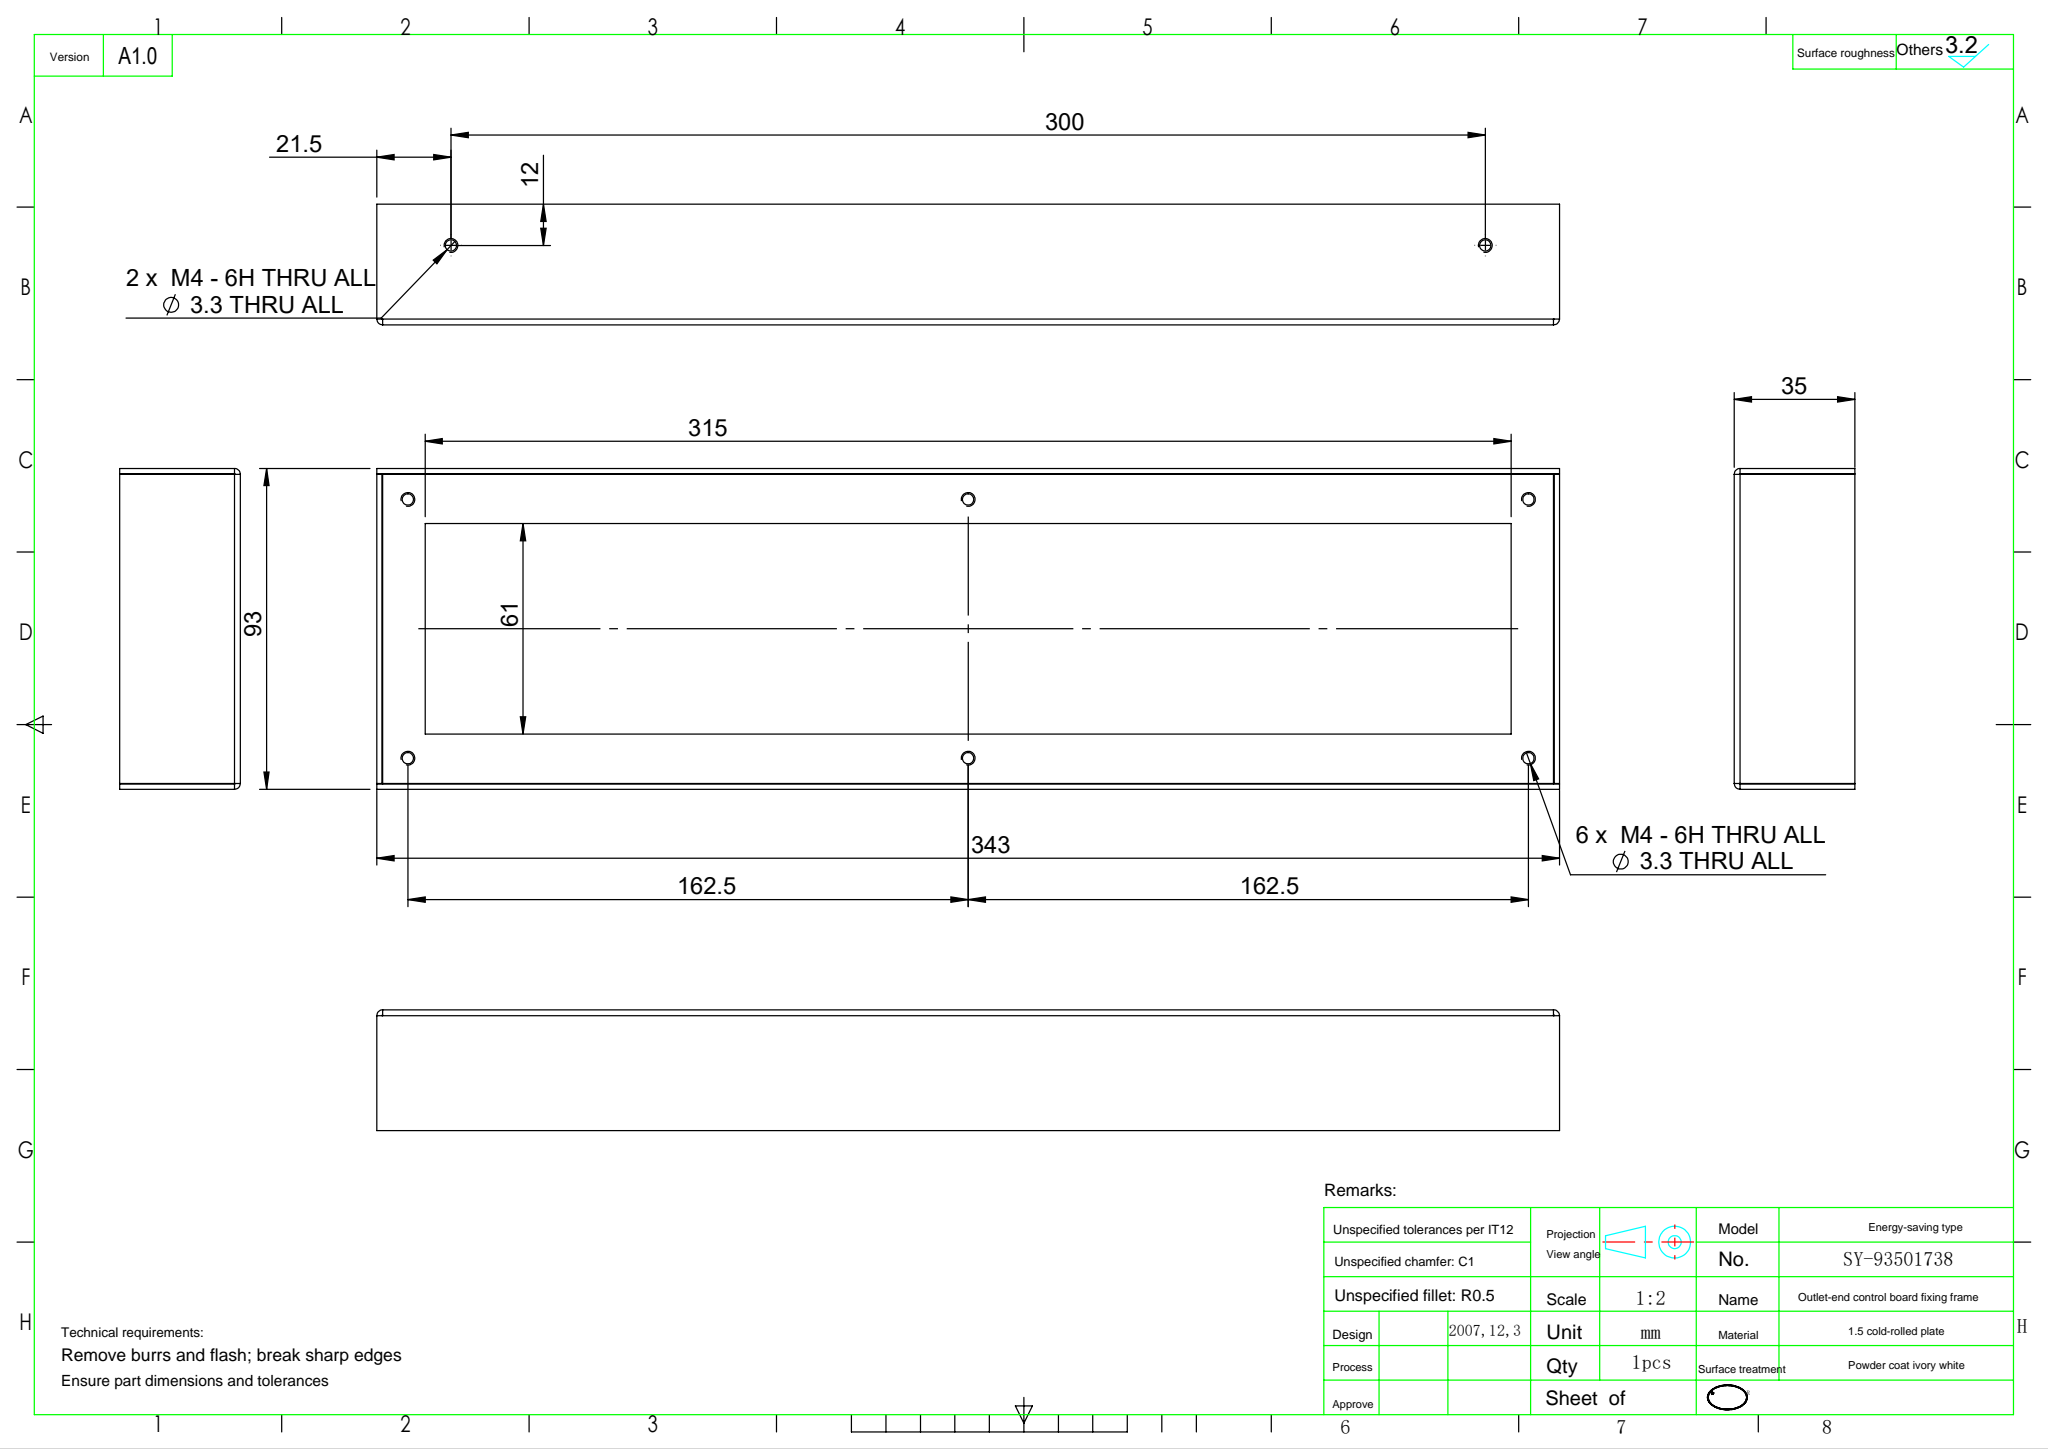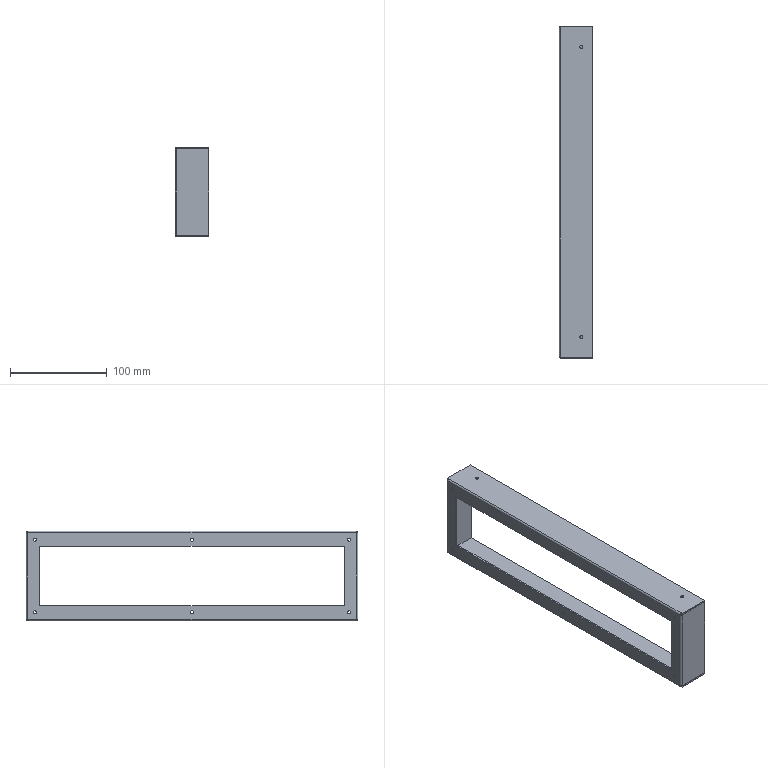Part | SolidWorks | features EdgeFlange 2, HoleWzd 2, ICE 2, FlatPattern 1, SMBaseFlange 1, SheetMetal 1 | 1 solid | 62 faces | box 35 x 343 x 93 mm | volume 61855 mm3 | plane 38 | cylinder 24 | commonest cylinder face diameters 3.3 x16 0.4 x4 3.4 x4